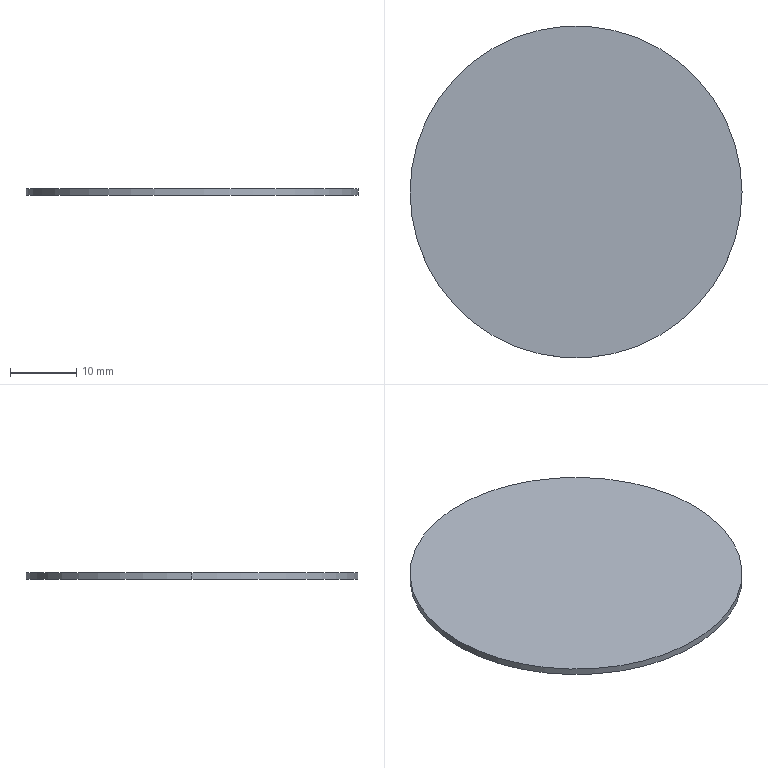Part | SolidWorks | features Extrusion 1 | 1 solid | 4 faces | box 50 x 50 x 1 mm | volume 1963 mm3 | cylinder 2 | plane 2 | commonest cylinder face diameters 50 x2
STEP:
#1=CARTESIAN_POINT('',(25.,0.,0.5));
#2=VERTEX_POINT('',#1);
#3=CARTESIAN_POINT('',(-25.,0.,0.5));
#4=VERTEX_POINT('',#3);
#5=CARTESIAN_POINT('',(0.,0.,0.5));
#6=DIRECTION('',(0.,0.,1.));
#7=DIRECTION('',(1.,0.,0.));
#8=AXIS2_PLACEMENT_3D('',#5,#6,#7);
#9=CIRCLE('',#8,25.);
#10=EDGE_CURVE('',#2,#4,#9,.T.);
#11=ORIENTED_EDGE('',*,*,#10,.F.);
#12=CARTESIAN_POINT('',(25.,0.,-0.5));
#13=VERTEX_POINT('',#12);
#14=CARTESIAN_POINT('',(25.,0.,0.5));
#15=DIRECTION('',(0.,0.,-1.));
#16=VECTOR('',#15,1000.);
#17=LINE('',#14,#16);
#18=EDGE_CURVE('',#2,#13,#17,.T.);
#19=ORIENTED_EDGE('',*,*,#18,.T.);
#20=CARTESIAN_POINT('',(-25.,0.,-0.5));
#21=VERTEX_POINT('',#20);
#22=CARTESIAN_POINT('',(0.,0.,-0.5));
#23=DIRECTION('',(0.,0.,1.));
#24=DIRECTION('',(1.,0.,0.));
#25=AXIS2_PLACEMENT_3D('',#22,#23,#24);
#26=CIRCLE('',#25,25.);
#27=EDGE_CURVE('',#13,#21,#26,.T.);
#28=ORIENTED_EDGE('',*,*,#27,.T.);
#29=CARTESIAN_POINT('',(-25.,0.,0.5));
#30=DIRECTION('',(0.,0.,-1.));
#31=VECTOR('',#30,1000.);
#32=LINE('',#29,#31);
#33=EDGE_CURVE('',#4,#21,#32,.T.);
#34=ORIENTED_EDGE('',*,*,#33,.F.);
#35=EDGE_LOOP('',(#11,#19,#28,#34));
#36=FACE_OUTER_BOUND('',#35,.T.);
#37=CARTESIAN_POINT('',(0.,0.,0.5));
#38=DIRECTION('',(0.,0.,-1.));
#39=DIRECTION('',(-1.,0.,0.));
#40=AXIS2_PLACEMENT_3D('',#37,#38,#39);
#41=CYLINDRICAL_SURFACE('',#40,25.);
#42=ADVANCED_FACE('',(#36),#41,.T.);
#43=ORIENTED_EDGE('',*,*,#18,.F.);
#44=CARTESIAN_POINT('',(0.,0.,0.5));
#45=DIRECTION('',(0.,0.,1.));
#46=DIRECTION('',(1.,0.,0.));
#47=AXIS2_PLACEMENT_3D('',#44,#45,#46);
#48=CIRCLE('',#47,25.);
#49=EDGE_CURVE('',#4,#2,#48,.T.);
#50=ORIENTED_EDGE('',*,*,#49,.F.);
#51=ORIENTED_EDGE('',*,*,#33,.T.);
#52=CARTESIAN_POINT('',(0.,0.,-0.5));
#53=DIRECTION('',(0.,0.,1.));
#54=DIRECTION('',(1.,0.,0.));
#55=AXIS2_PLACEMENT_3D('',#52,#53,#54);
#56=CIRCLE('',#55,25.);
#57=EDGE_CURVE('',#21,#13,#56,.T.);
#58=ORIENTED_EDGE('',*,*,#57,.T.);
#59=EDGE_LOOP('',(#43,#50,#51,#58));
#60=FACE_OUTER_BOUND('',#59,.T.);
#61=CARTESIAN_POINT('',(0.,0.,0.5));
#62=DIRECTION('',(0.,0.,-1.));
#63=DIRECTION('',(-1.,0.,0.));
#64=AXIS2_PLACEMENT_3D('',#61,#62,#63);
#65=CYLINDRICAL_SURFACE('',#64,25.);
#66=ADVANCED_FACE('',(#60),#65,.T.);
#67=ORIENTED_EDGE('',*,*,#49,.T.);
#68=ORIENTED_EDGE('',*,*,#10,.T.);
#69=EDGE_LOOP('',(#67,#68));
#70=FACE_OUTER_BOUND('',#69,.T.);
#71=CARTESIAN_POINT('',(0.,0.,0.5));
#72=DIRECTION('',(0.,0.,1.));
#73=DIRECTION('',(1.,0.,0.));
#74=AXIS2_PLACEMENT_3D('',#71,#72,#73);
#75=PLANE('',#74);
#76=ADVANCED_FACE('',(#70),#75,.T.);
#77=ORIENTED_EDGE('',*,*,#57,.F.);
#78=ORIENTED_EDGE('',*,*,#27,.F.);
#79=EDGE_LOOP('',(#77,#78));
#80=FACE_OUTER_BOUND('',#79,.T.);
#81=CARTESIAN_POINT('',(0.,0.,-0.5));
#82=DIRECTION('',(0.,0.,1.));
#83=DIRECTION('',(1.,0.,0.));
#84=AXIS2_PLACEMENT_3D('',#81,#82,#83);
#85=PLANE('',#84);
#86=ADVANCED_FACE('',(#80),#85,.F.);
#87=CLOSED_SHELL('',(#42,#66,#76,#86));
#88=MANIFOLD_SOLID_BREP('',#87);
#89=CARTESIAN_POINT('',(0.,0.,0.));
#90=DIRECTION('',(0.,0.,1.));
#91=DIRECTION('',(1.,0.,0.));
#92=AXIS2_PLACEMENT_3D('',#89,#90,#91);
#93=(LENGTH_UNIT()NAMED_UNIT(*)SI_UNIT(.MILLI.,.METRE.));
#94=UNCERTAINTY_MEASURE_WITH_UNIT(LENGTH_MEASURE(0.00001),#93,'','');
#95=(NAMED_UNIT(*)PLANE_ANGLE_UNIT()SI_UNIT($,.RADIAN.));
#96=(NAMED_UNIT(*)SI_UNIT($,.STERADIAN.)SOLID_ANGLE_UNIT());
#97=(GEOMETRIC_REPRESENTATION_CONTEXT(3)GLOBAL_UNCERTAINTY_ASSIGNED_CONTEXT((#94))GLOBAL_UNIT_ASSIGNED_CONTEXT((#93,#95,#96))REPRESENTATION_CONTEXT('',''));
#98=ADVANCED_BREP_SHAPE_REPRESENTATION('',(#88,#92),#97);